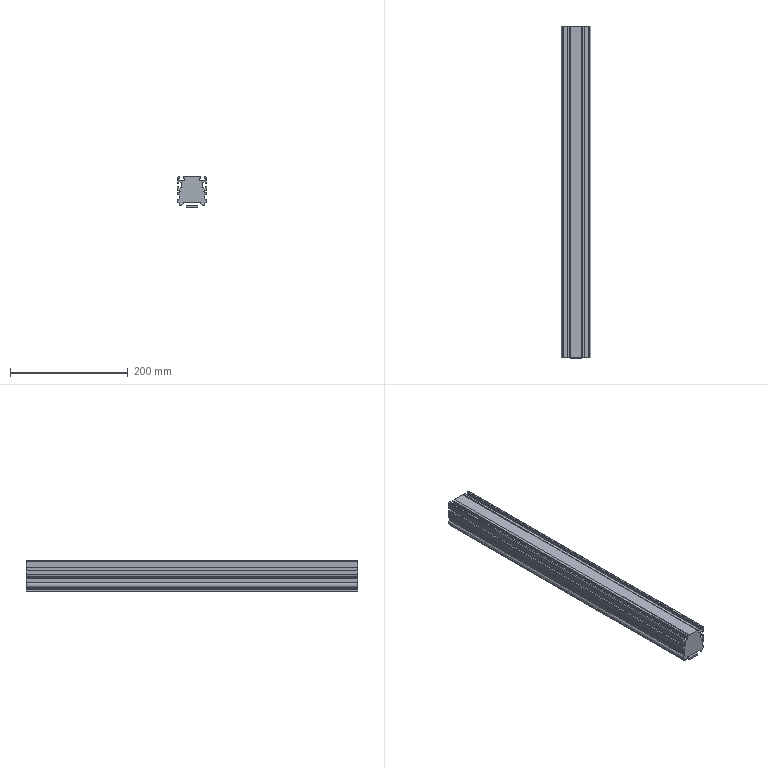Part | STEP file | Copy of 50-2016 profile^K50A-1H20-S(formula driven)-L1200 right | 2 solids | 143 faces | box 50 x 565 x 52.45 mm | volume 1145333 mm3 | plane 72 | cylinder 71 | commonest cylinder face diameters 0.4 x58 4.2 x6 4 x5 8 x2